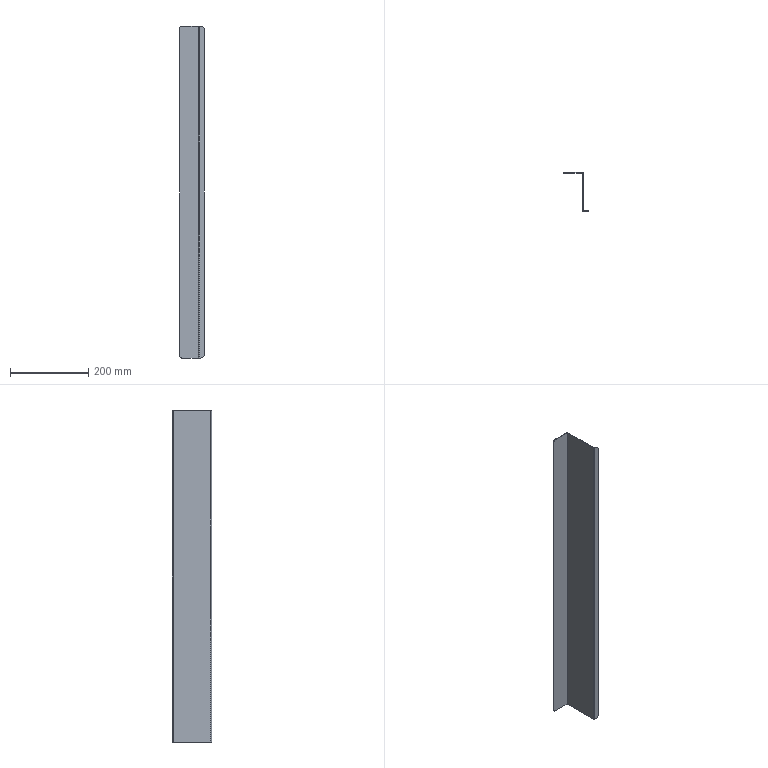Part | STEP file | HJDX-301 | 1 solid | 18 faces | box 63.5 x 100 x 850 mm | volume 205101 mm3 | plane 10 | cylinder 8 | commonest cylinder face diameters 1 x2 4 x2 10 x2 20 x2
STEP:
#1=CARTESIAN_POINT('',(-1.5,48.,-425.));
#2=VERTEX_POINT('',#1);
#3=CARTESIAN_POINT('',(-1.5,-48.,-425.));
#4=VERTEX_POINT('',#3);
#5=CARTESIAN_POINT('',(-1.5,0.,-425.));
#6=DIRECTION('',(0.,-1.,0.));
#7=VECTOR('',#6,1000.);
#8=LINE('',#5,#7);
#9=EDGE_CURVE('',#2,#4,#8,.T.);
#10=ORIENTED_EDGE('',*,*,#9,.T.);
#11=CARTESIAN_POINT('',(-1.5,-48.,425.));
#12=VERTEX_POINT('',#11);
#13=CARTESIAN_POINT('',(-1.5,-48.,0.));
#14=DIRECTION('',(0.,0.,1.));
#15=VECTOR('',#14,1000.);
#16=LINE('',#13,#15);
#17=EDGE_CURVE('',#4,#12,#16,.T.);
#18=ORIENTED_EDGE('',*,*,#17,.T.);
#19=CARTESIAN_POINT('',(-1.5,48.,425.));
#20=VERTEX_POINT('',#19);
#21=CARTESIAN_POINT('',(-1.5,0.,425.));
#22=DIRECTION('',(0.,1.,0.));
#23=VECTOR('',#22,1000.);
#24=LINE('',#21,#23);
#25=EDGE_CURVE('',#12,#20,#24,.T.);
#26=ORIENTED_EDGE('',*,*,#25,.T.);
#27=CARTESIAN_POINT('',(-1.5,48.,0.));
#28=DIRECTION('',(0.,0.,-1.));
#29=VECTOR('',#28,1000.);
#30=LINE('',#27,#29);
#31=EDGE_CURVE('',#20,#2,#30,.T.);
#32=ORIENTED_EDGE('',*,*,#31,.T.);
#33=EDGE_LOOP('',(#10,#18,#26,#32));
#34=FACE_OUTER_BOUND('',#33,.T.);
#35=CARTESIAN_POINT('',(-1.5,0.,0.));
#36=DIRECTION('',(-1.,0.,0.));
#37=DIRECTION('',(0.,0.,1.));
#38=AXIS2_PLACEMENT_3D('',#35,#36,#37);
#39=PLANE('',#38);
#40=ADVANCED_FACE('',(#34),#39,.T.);
#41=CARTESIAN_POINT('',(0.5,-50.,-425.));
#42=VERTEX_POINT('',#41);
#43=CARTESIAN_POINT('',(0.5,-50.,425.));
#44=VERTEX_POINT('',#43);
#45=CARTESIAN_POINT('',(0.5,-50.,-425.));
#46=DIRECTION('',(0.,0.,1.));
#47=VECTOR('',#46,1000.);
#48=LINE('',#45,#47);
#49=EDGE_CURVE('',#42,#44,#48,.T.);
#50=ORIENTED_EDGE('',*,*,#49,.T.);
#51=CARTESIAN_POINT('',(0.5,-48.,425.));
#52=DIRECTION('',(0.,0.,-1.));
#53=DIRECTION('',(-1.,0.,0.));
#54=AXIS2_PLACEMENT_3D('',#51,#52,#53);
#55=CIRCLE('',#54,2.);
#56=EDGE_CURVE('',#44,#12,#55,.T.);
#57=ORIENTED_EDGE('',*,*,#56,.T.);
#58=ORIENTED_EDGE('',*,*,#17,.F.);
#59=CARTESIAN_POINT('',(0.5,-48.,-425.));
#60=DIRECTION('',(0.,0.,1.));
#61=DIRECTION('',(-1.,0.,0.));
#62=AXIS2_PLACEMENT_3D('',#59,#60,#61);
#63=CIRCLE('',#62,2.);
#64=EDGE_CURVE('',#4,#42,#63,.T.);
#65=ORIENTED_EDGE('',*,*,#64,.T.);
#66=EDGE_LOOP('',(#50,#57,#58,#65));
#67=FACE_OUTER_BOUND('',#66,.T.);
#68=CARTESIAN_POINT('',(0.5,-48.,-425.));
#69=DIRECTION('',(0.,0.,-1.));
#70=DIRECTION('',(-1.,0.,0.));
#71=AXIS2_PLACEMENT_3D('',#68,#69,#70);
#72=CYLINDRICAL_SURFACE('',#71,2.);
#73=ADVANCED_FACE('',(#67),#72,.T.);
#74=CARTESIAN_POINT('',(0.,48.,-425.));
#75=VERTEX_POINT('',#74);
#76=CARTESIAN_POINT('',(0.,-48.,-425.));
#77=VERTEX_POINT('',#76);
#78=CARTESIAN_POINT('',(0.,-50.,-425.));
#79=DIRECTION('',(0.,-1.,0.));
#80=VECTOR('',#79,1000.);
#81=LINE('',#78,#80);
#82=EDGE_CURVE('',#75,#77,#81,.T.);
#83=ORIENTED_EDGE('',*,*,#82,.T.);
#84=CARTESIAN_POINT('',(0.5,-48.5,-425.));
#85=VERTEX_POINT('',#84);
#86=CARTESIAN_POINT('',(0.5,-48.,-425.));
#87=DIRECTION('',(0.,0.,1.));
#88=DIRECTION('',(-1.,0.,0.));
#89=AXIS2_PLACEMENT_3D('',#86,#87,#88);
#90=CIRCLE('',#89,0.5);
#91=EDGE_CURVE('',#77,#85,#90,.T.);
#92=ORIENTED_EDGE('',*,*,#91,.T.);
#93=CARTESIAN_POINT('',(3.5,-48.5,-425.));
#94=VERTEX_POINT('',#93);
#95=CARTESIAN_POINT('',(13.5,-48.5,-425.));
#96=DIRECTION('',(-1.,0.,0.));
#97=VECTOR('',#96,1000.);
#98=LINE('',#95,#97);
#99=EDGE_CURVE('',#94,#85,#98,.T.);
#100=ORIENTED_EDGE('',*,*,#99,.F.);
#101=CARTESIAN_POINT('',(3.5,-50.,-425.));
#102=VERTEX_POINT('',#101);
#103=CARTESIAN_POINT('',(3.5,-50.,-425.));
#104=DIRECTION('',(0.,1.,0.));
#105=VECTOR('',#104,1000.);
#106=LINE('',#103,#105);
#107=EDGE_CURVE('',#102,#94,#106,.T.);
#108=ORIENTED_EDGE('',*,*,#107,.F.);
#109=CARTESIAN_POINT('',(0.,-50.,-425.));
#110=DIRECTION('',(-1.,0.,0.));
#111=VECTOR('',#110,1000.);
#112=LINE('',#109,#111);
#113=EDGE_CURVE('',#102,#42,#112,.T.);
#114=ORIENTED_EDGE('',*,*,#113,.T.);
#115=ORIENTED_EDGE('',*,*,#64,.F.);
#116=ORIENTED_EDGE('',*,*,#9,.F.);
#117=CARTESIAN_POINT('',(-2.,48.5,-425.));
#118=VERTEX_POINT('',#117);
#119=CARTESIAN_POINT('',(-2.,48.,-425.));
#120=DIRECTION('',(0.,0.,-1.));
#121=DIRECTION('',(-1.,0.,0.));
#122=AXIS2_PLACEMENT_3D('',#119,#120,#121);
#123=CIRCLE('',#122,0.5);
#124=EDGE_CURVE('',#118,#2,#123,.T.);
#125=ORIENTED_EDGE('',*,*,#124,.F.);
#126=CARTESIAN_POINT('',(-45.,48.5,-425.));
#127=VERTEX_POINT('',#126);
#128=CARTESIAN_POINT('',(0.,48.5,-425.));
#129=DIRECTION('',(-1.,0.,0.));
#130=VECTOR('',#129,1000.);
#131=LINE('',#128,#130);
#132=EDGE_CURVE('',#118,#127,#131,.T.);
#133=ORIENTED_EDGE('',*,*,#132,.T.);
#134=CARTESIAN_POINT('',(-45.,50.,-425.));
#135=VERTEX_POINT('',#134);
#136=CARTESIAN_POINT('',(-45.,50.,-425.));
#137=DIRECTION('',(0.,-1.,0.));
#138=VECTOR('',#137,1000.);
#139=LINE('',#136,#138);
#140=EDGE_CURVE('',#135,#127,#139,.T.);
#141=ORIENTED_EDGE('',*,*,#140,.F.);
#142=CARTESIAN_POINT('',(-2.,50.,-425.));
#143=VERTEX_POINT('',#142);
#144=CARTESIAN_POINT('',(-1.5,50.,-425.));
#145=DIRECTION('',(1.,0.,0.));
#146=VECTOR('',#145,1000.);
#147=LINE('',#144,#146);
#148=EDGE_CURVE('',#135,#143,#147,.T.);
#149=ORIENTED_EDGE('',*,*,#148,.T.);
#150=CARTESIAN_POINT('',(-2.,48.,-425.));
#151=DIRECTION('',(0.,0.,1.));
#152=DIRECTION('',(-1.,0.,0.));
#153=AXIS2_PLACEMENT_3D('',#150,#151,#152);
#154=CIRCLE('',#153,2.);
#155=EDGE_CURVE('',#75,#143,#154,.T.);
#156=ORIENTED_EDGE('',*,*,#155,.F.);
#157=EDGE_LOOP('',(#83,#92,#100,#108,#114,#115,#116,#125,#133,#141,#149,#156));
#158=FACE_OUTER_BOUND('',#157,.T.);
#159=CARTESIAN_POINT('',(-1.5,-50.,-425.));
#160=DIRECTION('',(0.,0.,-1.));
#161=DIRECTION('',(-1.,0.,0.));
#162=AXIS2_PLACEMENT_3D('',#159,#160,#161);
#163=PLANE('',#162);
#164=ADVANCED_FACE('',(#158),#163,.T.);
#165=CARTESIAN_POINT('',(-2.,48.5,425.));
#166=VERTEX_POINT('',#165);
#167=CARTESIAN_POINT('',(-2.,48.,425.));
#168=DIRECTION('',(0.,0.,-1.));
#169=DIRECTION('',(-1.,0.,0.));
#170=AXIS2_PLACEMENT_3D('',#167,#168,#169);
#171=CIRCLE('',#170,0.5);
#172=EDGE_CURVE('',#166,#20,#171,.T.);
#173=ORIENTED_EDGE('',*,*,#172,.F.);
#174=CARTESIAN_POINT('',(-2.,48.5,-425.));
#175=DIRECTION('',(0.,0.,1.));
#176=VECTOR('',#175,1000.);
#177=LINE('',#174,#176);
#178=EDGE_CURVE('',#118,#166,#177,.T.);
#179=ORIENTED_EDGE('',*,*,#178,.F.);
#180=ORIENTED_EDGE('',*,*,#124,.T.);
#181=ORIENTED_EDGE('',*,*,#31,.F.);
#182=EDGE_LOOP('',(#173,#179,#180,#181));
#183=FACE_OUTER_BOUND('',#182,.T.);
#184=CARTESIAN_POINT('',(-2.,48.,-425.));
#185=DIRECTION('',(0.,0.,-1.));
#186=DIRECTION('',(-1.,0.,0.));
#187=AXIS2_PLACEMENT_3D('',#184,#185,#186);
#188=CYLINDRICAL_SURFACE('',#187,0.5);
#189=ADVANCED_FACE('',(#183),#188,.F.);
#190=ORIENTED_EDGE('',*,*,#25,.F.);
#191=ORIENTED_EDGE('',*,*,#56,.F.);
#192=CARTESIAN_POINT('',(3.5,-50.,425.));
#193=VERTEX_POINT('',#192);
#194=CARTESIAN_POINT('',(0.,-50.,425.));
#195=DIRECTION('',(1.,0.,0.));
#196=VECTOR('',#195,1000.);
#197=LINE('',#194,#196);
#198=EDGE_CURVE('',#44,#193,#197,.T.);
#199=ORIENTED_EDGE('',*,*,#198,.T.);
#200=CARTESIAN_POINT('',(3.5,-48.5,425.));
#201=VERTEX_POINT('',#200);
#202=CARTESIAN_POINT('',(3.5,-50.,425.));
#203=DIRECTION('',(0.,-1.,0.));
#204=VECTOR('',#203,1000.);
#205=LINE('',#202,#204);
#206=EDGE_CURVE('',#201,#193,#205,.T.);
#207=ORIENTED_EDGE('',*,*,#206,.F.);
#208=CARTESIAN_POINT('',(0.5,-48.5,425.));
#209=VERTEX_POINT('',#208);
#210=CARTESIAN_POINT('',(0.,-48.5,425.));
#211=DIRECTION('',(1.,0.,0.));
#212=VECTOR('',#211,1000.);
#213=LINE('',#210,#212);
#214=EDGE_CURVE('',#209,#201,#213,.T.);
#215=ORIENTED_EDGE('',*,*,#214,.F.);
#216=CARTESIAN_POINT('',(0.,-48.,425.));
#217=VERTEX_POINT('',#216);
#218=CARTESIAN_POINT('',(0.5,-48.,425.));
#219=DIRECTION('',(0.,0.,-1.));
#220=DIRECTION('',(-1.,0.,0.));
#221=AXIS2_PLACEMENT_3D('',#218,#219,#220);
#222=CIRCLE('',#221,0.5);
#223=EDGE_CURVE('',#209,#217,#222,.T.);
#224=ORIENTED_EDGE('',*,*,#223,.T.);
#225=CARTESIAN_POINT('',(0.,48.,425.));
#226=VERTEX_POINT('',#225);
#227=CARTESIAN_POINT('',(0.,-50.,425.));
#228=DIRECTION('',(0.,1.,0.));
#229=VECTOR('',#228,1000.);
#230=LINE('',#227,#229);
#231=EDGE_CURVE('',#217,#226,#230,.T.);
#232=ORIENTED_EDGE('',*,*,#231,.T.);
#233=CARTESIAN_POINT('',(-2.,50.,425.));
#234=VERTEX_POINT('',#233);
#235=CARTESIAN_POINT('',(-2.,48.,425.));
#236=DIRECTION('',(0.,0.,-1.));
#237=DIRECTION('',(-1.,0.,0.));
#238=AXIS2_PLACEMENT_3D('',#235,#236,#237);
#239=CIRCLE('',#238,2.);
#240=EDGE_CURVE('',#234,#226,#239,.T.);
#241=ORIENTED_EDGE('',*,*,#240,.F.);
#242=CARTESIAN_POINT('',(-45.,50.,425.));
#243=VERTEX_POINT('',#242);
#244=CARTESIAN_POINT('',(-50.,50.,425.));
#245=DIRECTION('',(-1.,0.,0.));
#246=VECTOR('',#245,1000.);
#247=LINE('',#244,#246);
#248=EDGE_CURVE('',#234,#243,#247,.T.);
#249=ORIENTED_EDGE('',*,*,#248,.T.);
#250=CARTESIAN_POINT('',(-45.,48.5,425.));
#251=VERTEX_POINT('',#250);
#252=CARTESIAN_POINT('',(-45.,50.,425.));
#253=DIRECTION('',(0.,-1.,0.));
#254=VECTOR('',#253,1000.);
#255=LINE('',#252,#254);
#256=EDGE_CURVE('',#243,#251,#255,.T.);
#257=ORIENTED_EDGE('',*,*,#256,.T.);
#258=CARTESIAN_POINT('',(0.,48.5,425.));
#259=DIRECTION('',(1.,0.,0.));
#260=VECTOR('',#259,1000.);
#261=LINE('',#258,#260);
#262=EDGE_CURVE('',#251,#166,#261,.T.);
#263=ORIENTED_EDGE('',*,*,#262,.T.);
#264=ORIENTED_EDGE('',*,*,#172,.T.);
#265=EDGE_LOOP('',(#190,#191,#199,#207,#215,#224,#232,#241,#249,#257,#263,#264));
#266=FACE_OUTER_BOUND('',#265,.T.);
#267=CARTESIAN_POINT('',(-1.5,-50.,425.));
#268=DIRECTION('',(0.,0.,1.));
#269=DIRECTION('',(1.,0.,0.));
#270=AXIS2_PLACEMENT_3D('',#267,#268,#269);
#271=PLANE('',#270);
#272=ADVANCED_FACE('',(#266),#271,.T.);
#273=CARTESIAN_POINT('',(13.5,-50.,-415.));
#274=VERTEX_POINT('',#273);
#275=CARTESIAN_POINT('',(3.5,-50.,-415.));
#276=DIRECTION('',(0.,1.,0.));
#277=DIRECTION('',(-1.,0.,0.));
#278=AXIS2_PLACEMENT_3D('',#275,#276,#277);
#279=CIRCLE('',#278,10.);
#280=EDGE_CURVE('',#274,#102,#279,.T.);
#281=ORIENTED_EDGE('',*,*,#280,.F.);
#282=CARTESIAN_POINT('',(13.5,-50.,415.));
#283=VERTEX_POINT('',#282);
#284=CARTESIAN_POINT('',(13.5,-50.,0.));
#285=DIRECTION('',(0.,0.,-1.));
#286=VECTOR('',#285,1000.);
#287=LINE('',#284,#286);
#288=EDGE_CURVE('',#283,#274,#287,.T.);
#289=ORIENTED_EDGE('',*,*,#288,.F.);
#290=CARTESIAN_POINT('',(3.5,-50.,415.));
#291=DIRECTION('',(0.,1.,0.));
#292=DIRECTION('',(-1.,0.,0.));
#293=AXIS2_PLACEMENT_3D('',#290,#291,#292);
#294=CIRCLE('',#293,10.);
#295=EDGE_CURVE('',#193,#283,#294,.T.);
#296=ORIENTED_EDGE('',*,*,#295,.F.);
#297=ORIENTED_EDGE('',*,*,#198,.F.);
#298=ORIENTED_EDGE('',*,*,#49,.F.);
#299=ORIENTED_EDGE('',*,*,#113,.F.);
#300=EDGE_LOOP('',(#281,#289,#296,#297,#298,#299));
#301=FACE_OUTER_BOUND('',#300,.T.);
#302=CARTESIAN_POINT('',(0.,-50.,0.));
#303=DIRECTION('',(0.,1.,0.));
#304=DIRECTION('',(-1.,0.,0.));
#305=AXIS2_PLACEMENT_3D('',#302,#303,#304);
#306=PLANE('',#305);
#307=ADVANCED_FACE('',(#301),#306,.F.);
#308=ORIENTED_EDGE('',*,*,#231,.F.);
#309=CARTESIAN_POINT('',(0.,-48.,0.));
#310=DIRECTION('',(0.,0.,1.));
#311=VECTOR('',#310,1000.);
#312=LINE('',#309,#311);
#313=EDGE_CURVE('',#77,#217,#312,.T.);
#314=ORIENTED_EDGE('',*,*,#313,.F.);
#315=ORIENTED_EDGE('',*,*,#82,.F.);
#316=CARTESIAN_POINT('',(0.,48.,0.));
#317=DIRECTION('',(0.,0.,-1.));
#318=VECTOR('',#317,1000.);
#319=LINE('',#316,#318);
#320=EDGE_CURVE('',#226,#75,#319,.T.);
#321=ORIENTED_EDGE('',*,*,#320,.F.);
#322=EDGE_LOOP('',(#308,#314,#315,#321));
#323=FACE_OUTER_BOUND('',#322,.T.);
#324=CARTESIAN_POINT('',(0.,0.,0.));
#325=DIRECTION('',(-1.,0.,0.));
#326=DIRECTION('',(0.,0.,1.));
#327=AXIS2_PLACEMENT_3D('',#324,#325,#326);
#328=PLANE('',#327);
#329=ADVANCED_FACE('',(#323),#328,.F.);
#330=CARTESIAN_POINT('',(-50.,48.5,-420.));
#331=VERTEX_POINT('',#330);
#332=CARTESIAN_POINT('',(-45.,48.5,-420.));
#333=DIRECTION('',(0.,1.,0.));
#334=DIRECTION('',(1.,0.,0.));
#335=AXIS2_PLACEMENT_3D('',#332,#333,#334);
#336=CIRCLE('',#335,5.);
#337=EDGE_CURVE('',#127,#331,#336,.T.);
#338=ORIENTED_EDGE('',*,*,#337,.F.);
#339=ORIENTED_EDGE('',*,*,#132,.F.);
#340=ORIENTED_EDGE('',*,*,#178,.T.);
#341=ORIENTED_EDGE('',*,*,#262,.F.);
#342=CARTESIAN_POINT('',(-50.,48.5,420.));
#343=VERTEX_POINT('',#342);
#344=CARTESIAN_POINT('',(-45.,48.5,420.));
#345=DIRECTION('',(0.,1.,0.));
#346=DIRECTION('',(1.,0.,0.));
#347=AXIS2_PLACEMENT_3D('',#344,#345,#346);
#348=CIRCLE('',#347,5.);
#349=EDGE_CURVE('',#343,#251,#348,.T.);
#350=ORIENTED_EDGE('',*,*,#349,.F.);
#351=CARTESIAN_POINT('',(-50.,48.5,0.));
#352=DIRECTION('',(0.,0.,1.));
#353=VECTOR('',#352,1000.);
#354=LINE('',#351,#353);
#355=EDGE_CURVE('',#331,#343,#354,.T.);
#356=ORIENTED_EDGE('',*,*,#355,.F.);
#357=EDGE_LOOP('',(#338,#339,#340,#341,#350,#356));
#358=FACE_OUTER_BOUND('',#357,.T.);
#359=CARTESIAN_POINT('',(0.,48.5,0.));
#360=DIRECTION('',(0.,1.,0.));
#361=DIRECTION('',(-1.,0.,0.));
#362=AXIS2_PLACEMENT_3D('',#359,#360,#361);
#363=PLANE('',#362);
#364=ADVANCED_FACE('',(#358),#363,.F.);
#365=CARTESIAN_POINT('',(13.5,-48.5,-415.));
#366=VERTEX_POINT('',#365);
#367=CARTESIAN_POINT('',(3.5,-48.5,-415.));
#368=DIRECTION('',(0.,-1.,0.));
#369=DIRECTION('',(-1.,0.,0.));
#370=AXIS2_PLACEMENT_3D('',#367,#368,#369);
#371=CIRCLE('',#370,10.);
#372=EDGE_CURVE('',#94,#366,#371,.T.);
#373=ORIENTED_EDGE('',*,*,#372,.T.);
#374=CARTESIAN_POINT('',(13.5,-50.,-415.));
#375=DIRECTION('',(0.,-1.,0.));
#376=VECTOR('',#375,1000.);
#377=LINE('',#374,#376);
#378=EDGE_CURVE('',#366,#274,#377,.T.);
#379=ORIENTED_EDGE('',*,*,#378,.T.);
#380=ORIENTED_EDGE('',*,*,#280,.T.);
#381=ORIENTED_EDGE('',*,*,#107,.T.);
#382=EDGE_LOOP('',(#373,#379,#380,#381));
#383=FACE_OUTER_BOUND('',#382,.T.);
#384=CARTESIAN_POINT('',(3.5,-50.,-415.));
#385=DIRECTION('',(0.,1.,0.));
#386=DIRECTION('',(-1.,0.,0.));
#387=AXIS2_PLACEMENT_3D('',#384,#385,#386);
#388=CYLINDRICAL_SURFACE('',#387,10.);
#389=ADVANCED_FACE('',(#383),#388,.T.);
#390=ORIENTED_EDGE('',*,*,#378,.F.);
#391=CARTESIAN_POINT('',(13.5,-48.5,415.));
#392=VERTEX_POINT('',#391);
#393=CARTESIAN_POINT('',(13.5,-48.5,425.));
#394=DIRECTION('',(0.,0.,-1.));
#395=VECTOR('',#394,1000.);
#396=LINE('',#393,#395);
#397=EDGE_CURVE('',#392,#366,#396,.T.);
#398=ORIENTED_EDGE('',*,*,#397,.F.);
#399=CARTESIAN_POINT('',(13.5,-50.,415.));
#400=DIRECTION('',(0.,1.,0.));
#401=VECTOR('',#400,1000.);
#402=LINE('',#399,#401);
#403=EDGE_CURVE('',#283,#392,#402,.T.);
#404=ORIENTED_EDGE('',*,*,#403,.F.);
#405=ORIENTED_EDGE('',*,*,#288,.T.);
#406=EDGE_LOOP('',(#390,#398,#404,#405));
#407=FACE_OUTER_BOUND('',#406,.T.);
#408=CARTESIAN_POINT('',(13.5,-50.,425.));
#409=DIRECTION('',(-1.,0.,0.));
#410=DIRECTION('',(0.,-1.,0.));
#411=AXIS2_PLACEMENT_3D('',#408,#409,#410);
#412=PLANE('',#411);
#413=ADVANCED_FACE('',(#407),#412,.F.);
#414=CARTESIAN_POINT('',(3.5,-48.5,415.));
#415=DIRECTION('',(0.,-1.,0.));
#416=DIRECTION('',(-1.,0.,0.));
#417=AXIS2_PLACEMENT_3D('',#414,#415,#416);
#418=CIRCLE('',#417,10.);
#419=EDGE_CURVE('',#392,#201,#418,.T.);
#420=ORIENTED_EDGE('',*,*,#419,.T.);
#421=ORIENTED_EDGE('',*,*,#206,.T.);
#422=ORIENTED_EDGE('',*,*,#295,.T.);
#423=ORIENTED_EDGE('',*,*,#403,.T.);
#424=EDGE_LOOP('',(#420,#421,#422,#423));
#425=FACE_OUTER_BOUND('',#424,.T.);
#426=CARTESIAN_POINT('',(3.5,-50.,415.));
#427=DIRECTION('',(0.,1.,0.));
#428=DIRECTION('',(-1.,0.,0.));
#429=AXIS2_PLACEMENT_3D('',#426,#427,#428);
#430=CYLINDRICAL_SURFACE('',#429,10.);
#431=ADVANCED_FACE('',(#425),#430,.T.);
#432=CARTESIAN_POINT('',(-2.,50.,-425.));
#433=DIRECTION('',(0.,0.,1.));
#434=VECTOR('',#433,1000.);
#435=LINE('',#432,#434);
#436=EDGE_CURVE('',#143,#234,#435,.T.);
#437=ORIENTED_EDGE('',*,*,#436,.T.);
#438=ORIENTED_EDGE('',*,*,#240,.T.);
#439=ORIENTED_EDGE('',*,*,#320,.T.);
#440=ORIENTED_EDGE('',*,*,#155,.T.);
#441=EDGE_LOOP('',(#437,#438,#439,#440));
#442=FACE_OUTER_BOUND('',#441,.T.);
#443=CARTESIAN_POINT('',(-2.,48.,-425.));
#444=DIRECTION('',(0.,0.,-1.));
#445=DIRECTION('',(-1.,0.,0.));
#446=AXIS2_PLACEMENT_3D('',#443,#444,#445);
#447=CYLINDRICAL_SURFACE('',#446,2.);
#448=ADVANCED_FACE('',(#442),#447,.T.);
#449=ORIENTED_EDGE('',*,*,#223,.F.);
#450=CARTESIAN_POINT('',(0.5,-48.5,-425.));
#451=DIRECTION('',(0.,0.,1.));
#452=VECTOR('',#451,1000.);
#453=LINE('',#450,#452);
#454=EDGE_CURVE('',#85,#209,#453,.T.);
#455=ORIENTED_EDGE('',*,*,#454,.F.);
#456=ORIENTED_EDGE('',*,*,#91,.F.);
#457=ORIENTED_EDGE('',*,*,#313,.T.);
#458=EDGE_LOOP('',(#449,#455,#456,#457));
#459=FACE_OUTER_BOUND('',#458,.T.);
#460=CARTESIAN_POINT('',(0.5,-48.,-425.));
#461=DIRECTION('',(0.,0.,-1.));
#462=DIRECTION('',(-1.,0.,0.));
#463=AXIS2_PLACEMENT_3D('',#460,#461,#462);
#464=CYLINDRICAL_SURFACE('',#463,0.5);
#465=ADVANCED_FACE('',(#459),#464,.F.);
#466=ORIENTED_EDGE('',*,*,#355,.T.);
#467=CARTESIAN_POINT('',(-50.,50.,420.));
#468=VERTEX_POINT('',#467);
#469=CARTESIAN_POINT('',(-50.,50.,420.));
#470=DIRECTION('',(0.,1.,0.));
#471=VECTOR('',#470,1000.);
#472=LINE('',#469,#471);
#473=EDGE_CURVE('',#343,#468,#472,.T.);
#474=ORIENTED_EDGE('',*,*,#473,.T.);
#475=CARTESIAN_POINT('',(-50.,50.,-420.));
#476=VERTEX_POINT('',#475);
#477=CARTESIAN_POINT('',(-50.,50.,-425.));
#478=DIRECTION('',(0.,0.,-1.));
#479=VECTOR('',#478,1000.);
#480=LINE('',#477,#479);
#481=EDGE_CURVE('',#468,#476,#480,.T.);
#482=ORIENTED_EDGE('',*,*,#481,.T.);
#483=CARTESIAN_POINT('',(-50.,50.,-420.));
#484=DIRECTION('',(0.,-1.,0.));
#485=VECTOR('',#484,1000.);
#486=LINE('',#483,#485);
#487=EDGE_CURVE('',#476,#331,#486,.T.);
#488=ORIENTED_EDGE('',*,*,#487,.T.);
#489=EDGE_LOOP('',(#466,#474,#482,#488));
#490=FACE_OUTER_BOUND('',#489,.T.);
#491=CARTESIAN_POINT('',(-50.,50.,-425.));
#492=DIRECTION('',(-1.,0.,0.));
#493=DIRECTION('',(0.,-1.,0.));
#494=AXIS2_PLACEMENT_3D('',#491,#492,#493);
#495=PLANE('',#494);
#496=ADVANCED_FACE('',(#490),#495,.T.);
#497=ORIENTED_EDGE('',*,*,#337,.T.);
#498=ORIENTED_EDGE('',*,*,#487,.F.);
#499=CARTESIAN_POINT('',(-45.,50.,-420.));
#500=DIRECTION('',(0.,-1.,0.));
#501=DIRECTION('',(1.,0.,0.));
#502=AXIS2_PLACEMENT_3D('',#499,#500,#501);
#503=CIRCLE('',#502,5.);
#504=EDGE_CURVE('',#476,#135,#503,.T.);
#505=ORIENTED_EDGE('',*,*,#504,.T.);
#506=ORIENTED_EDGE('',*,*,#140,.T.);
#507=EDGE_LOOP('',(#497,#498,#505,#506));
#508=FACE_OUTER_BOUND('',#507,.T.);
#509=CARTESIAN_POINT('',(-45.,50.,-420.));
#510=DIRECTION('',(0.,-1.,0.));
#511=DIRECTION('',(1.,0.,0.));
#512=AXIS2_PLACEMENT_3D('',#509,#510,#511);
#513=CYLINDRICAL_SURFACE('',#512,5.);
#514=ADVANCED_FACE('',(#508),#513,.T.);
#515=ORIENTED_EDGE('',*,*,#349,.T.);
#516=ORIENTED_EDGE('',*,*,#256,.F.);
#517=CARTESIAN_POINT('',(-45.,50.,420.));
#518=DIRECTION('',(0.,-1.,0.));
#519=DIRECTION('',(1.,0.,0.));
#520=AXIS2_PLACEMENT_3D('',#517,#518,#519);
#521=CIRCLE('',#520,5.);
#522=EDGE_CURVE('',#243,#468,#521,.T.);
#523=ORIENTED_EDGE('',*,*,#522,.T.);
#524=ORIENTED_EDGE('',*,*,#473,.F.);
#525=EDGE_LOOP('',(#515,#516,#523,#524));
#526=FACE_OUTER_BOUND('',#525,.T.);
#527=CARTESIAN_POINT('',(-45.,50.,420.));
#528=DIRECTION('',(0.,-1.,0.));
#529=DIRECTION('',(1.,0.,0.));
#530=AXIS2_PLACEMENT_3D('',#527,#528,#529);
#531=CYLINDRICAL_SURFACE('',#530,5.);
#532=ADVANCED_FACE('',(#526),#531,.T.);
#533=ORIENTED_EDGE('',*,*,#214,.T.);
#534=ORIENTED_EDGE('',*,*,#419,.F.);
#535=ORIENTED_EDGE('',*,*,#397,.T.);
#536=ORIENTED_EDGE('',*,*,#372,.F.);
#537=ORIENTED_EDGE('',*,*,#99,.T.);
#538=ORIENTED_EDGE('',*,*,#454,.T.);
#539=EDGE_LOOP('',(#533,#534,#535,#536,#537,#538));
#540=FACE_OUTER_BOUND('',#539,.T.);
#541=CARTESIAN_POINT('',(0.,-48.5,0.));
#542=DIRECTION('',(0.,1.,0.));
#543=DIRECTION('',(-1.,0.,0.));
#544=AXIS2_PLACEMENT_3D('',#541,#542,#543);
#545=PLANE('',#544);
#546=ADVANCED_FACE('',(#540),#545,.T.);
#547=ORIENTED_EDGE('',*,*,#248,.F.);
#548=ORIENTED_EDGE('',*,*,#436,.F.);
#549=ORIENTED_EDGE('',*,*,#148,.F.);
#550=ORIENTED_EDGE('',*,*,#504,.F.);
#551=ORIENTED_EDGE('',*,*,#481,.F.);
#552=ORIENTED_EDGE('',*,*,#522,.F.);
#553=EDGE_LOOP('',(#547,#548,#549,#550,#551,#552));
#554=FACE_OUTER_BOUND('',#553,.T.);
#555=CARTESIAN_POINT('',(0.,50.,0.));
#556=DIRECTION('',(0.,1.,0.));
#557=DIRECTION('',(-1.,0.,0.));
#558=AXIS2_PLACEMENT_3D('',#555,#556,#557);
#559=PLANE('',#558);
#560=ADVANCED_FACE('',(#554),#559,.T.);
#561=CLOSED_SHELL('',(#40,#73,#164,#189,#272,#307,#329,#364,#389,#413,#431,#448,#465,#496,#514,#532,#546,#560));
#562=MANIFOLD_SOLID_BREP('',#561);
#563=CARTESIAN_POINT('',(0.,0.,0.));
#564=DIRECTION('',(0.,0.,1.));
#565=DIRECTION('',(1.,0.,0.));
#566=AXIS2_PLACEMENT_3D('',#563,#564,#565);
#567=(LENGTH_UNIT()NAMED_UNIT(*)SI_UNIT(.MILLI.,.METRE.));
#568=UNCERTAINTY_MEASURE_WITH_UNIT(LENGTH_MEASURE(0.00001),#567,'','');
#569=(NAMED_UNIT(*)PLANE_ANGLE_UNIT()SI_UNIT($,.RADIAN.));
#570=(NAMED_UNIT(*)SI_UNIT($,.STERADIAN.)SOLID_ANGLE_UNIT());
#571=(GEOMETRIC_REPRESENTATION_CONTEXT(3)GLOBAL_UNCERTAINTY_ASSIGNED_CONTEXT((#568))GLOBAL_UNIT_ASSIGNED_CONTEXT((#567,#569,#570))REPRESENTATION_CONTEXT('',''));
#572=ADVANCED_BREP_SHAPE_REPRESENTATION('',(#562,#566),#571);